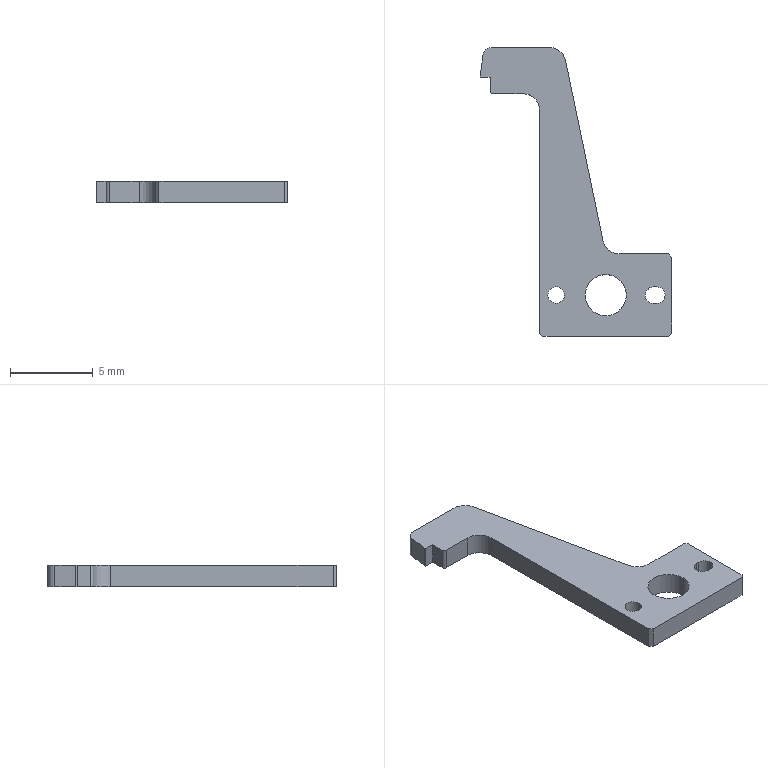Part | SolidWorks | features ICE 4, Fillet 3, Chamfer 1, Extrusion 1 | 1 solid | 30 faces | box 11.6 x 17.5 x 1.3 mm | volume 99.407 mm3 | plane 18 | cylinder 12 | commonest cylinder face diameters 1 x6 2 x3 2.5 x2 0.4 x1
STEP:
#1=CARTESIAN_POINT('',(5.4,-6.25,-0.65));
#2=VERTEX_POINT('',#1);
#3=CARTESIAN_POINT('',(4.9,-5.75,-0.65));
#4=VERTEX_POINT('',#3);
#5=CARTESIAN_POINT('',(4.9,-6.25,-0.65));
#6=DIRECTION('',(0.,0.,1.));
#7=DIRECTION('',(1.,0.,0.));
#8=AXIS2_PLACEMENT_3D('',#5,#6,#7);
#9=CIRCLE('',#8,0.5);
#10=EDGE_CURVE('',#2,#4,#9,.T.);
#11=ORIENTED_EDGE('',*,*,#10,.F.);
#12=CARTESIAN_POINT('',(5.4,-6.25,0.65));
#13=VERTEX_POINT('',#12);
#14=CARTESIAN_POINT('',(5.4,-6.25,-0.65));
#15=DIRECTION('',(0.,0.,1.));
#16=VECTOR('',#15,1000.);
#17=LINE('',#14,#16);
#18=EDGE_CURVE('',#2,#13,#17,.T.);
#19=ORIENTED_EDGE('',*,*,#18,.T.);
#20=CARTESIAN_POINT('',(4.9,-5.75,0.65));
#21=VERTEX_POINT('',#20);
#22=CARTESIAN_POINT('',(4.9,-6.25,0.65));
#23=DIRECTION('',(0.,0.,1.));
#24=DIRECTION('',(1.,0.,0.));
#25=AXIS2_PLACEMENT_3D('',#22,#23,#24);
#26=CIRCLE('',#25,0.5);
#27=EDGE_CURVE('',#13,#21,#26,.T.);
#28=ORIENTED_EDGE('',*,*,#27,.T.);
#29=CARTESIAN_POINT('',(4.9,-5.75,-0.65));
#30=DIRECTION('',(0.,0.,1.));
#31=VECTOR('',#30,1000.);
#32=LINE('',#29,#31);
#33=EDGE_CURVE('',#4,#21,#32,.T.);
#34=ORIENTED_EDGE('',*,*,#33,.F.);
#35=EDGE_LOOP('',(#11,#19,#28,#34));
#36=FACE_OUTER_BOUND('',#35,.T.);
#37=CARTESIAN_POINT('',(4.9,-6.25,-0.65));
#38=DIRECTION('',(0.,0.,1.));
#39=DIRECTION('',(1.,0.,0.));
#40=AXIS2_PLACEMENT_3D('',#37,#38,#39);
#41=CYLINDRICAL_SURFACE('',#40,0.5);
#42=ADVANCED_FACE('',(#36),#41,.F.);
#43=CARTESIAN_POINT('',(-1.7,-6.25,-0.65));
#44=VERTEX_POINT('',#43);
#45=CARTESIAN_POINT('',(-0.7,-6.25,-0.65));
#46=VERTEX_POINT('',#45);
#47=CARTESIAN_POINT('',(-1.2,-6.25,-0.65));
#48=DIRECTION('',(0.,0.,1.));
#49=DIRECTION('',(1.,0.,0.));
#50=AXIS2_PLACEMENT_3D('',#47,#48,#49);
#51=CIRCLE('',#50,0.5);
#52=EDGE_CURVE('',#44,#46,#51,.T.);
#53=ORIENTED_EDGE('',*,*,#52,.F.);
#54=CARTESIAN_POINT('',(-1.7,-6.25,0.65));
#55=VERTEX_POINT('',#54);
#56=CARTESIAN_POINT('',(-1.7,-6.25,-0.65));
#57=DIRECTION('',(0.,0.,1.));
#58=VECTOR('',#57,1000.);
#59=LINE('',#56,#58);
#60=EDGE_CURVE('',#44,#55,#59,.T.);
#61=ORIENTED_EDGE('',*,*,#60,.T.);
#62=CARTESIAN_POINT('',(-0.7,-6.25,0.65));
#63=VERTEX_POINT('',#62);
#64=CARTESIAN_POINT('',(-1.2,-6.25,0.65));
#65=DIRECTION('',(0.,0.,1.));
#66=DIRECTION('',(1.,0.,0.));
#67=AXIS2_PLACEMENT_3D('',#64,#65,#66);
#68=CIRCLE('',#67,0.5);
#69=EDGE_CURVE('',#55,#63,#68,.T.);
#70=ORIENTED_EDGE('',*,*,#69,.T.);
#71=CARTESIAN_POINT('',(-0.7,-6.25,-0.65));
#72=DIRECTION('',(0.,0.,1.));
#73=VECTOR('',#72,1000.);
#74=LINE('',#71,#73);
#75=EDGE_CURVE('',#46,#63,#74,.T.);
#76=ORIENTED_EDGE('',*,*,#75,.F.);
#77=EDGE_LOOP('',(#53,#61,#70,#76));
#78=FACE_OUTER_BOUND('',#77,.T.);
#79=CARTESIAN_POINT('',(-1.2,-6.25,-0.65));
#80=DIRECTION('',(0.,0.,1.));
#81=DIRECTION('',(1.,0.,0.));
#82=AXIS2_PLACEMENT_3D('',#79,#80,#81);
#83=CYLINDRICAL_SURFACE('',#82,0.5);
#84=ADVANCED_FACE('',(#78),#83,.F.);
#85=CARTESIAN_POINT('',(0.55,-6.25,-0.65));
#86=VERTEX_POINT('',#85);
#87=CARTESIAN_POINT('',(3.05,-6.25,-0.65));
#88=VERTEX_POINT('',#87);
#89=CARTESIAN_POINT('',(1.8,-6.25,-0.65));
#90=DIRECTION('',(0.,0.,1.));
#91=DIRECTION('',(1.,0.,0.));
#92=AXIS2_PLACEMENT_3D('',#89,#90,#91);
#93=CIRCLE('',#92,1.25);
#94=EDGE_CURVE('',#86,#88,#93,.T.);
#95=ORIENTED_EDGE('',*,*,#94,.F.);
#96=CARTESIAN_POINT('',(0.55,-6.25,0.65));
#97=VERTEX_POINT('',#96);
#98=CARTESIAN_POINT('',(0.55,-6.25,-0.65));
#99=DIRECTION('',(0.,0.,1.));
#100=VECTOR('',#99,1000.);
#101=LINE('',#98,#100);
#102=EDGE_CURVE('',#86,#97,#101,.T.);
#103=ORIENTED_EDGE('',*,*,#102,.T.);
#104=CARTESIAN_POINT('',(3.05,-6.25,0.65));
#105=VERTEX_POINT('',#104);
#106=CARTESIAN_POINT('',(1.8,-6.25,0.65));
#107=DIRECTION('',(0.,0.,1.));
#108=DIRECTION('',(1.,0.,0.));
#109=AXIS2_PLACEMENT_3D('',#106,#107,#108);
#110=CIRCLE('',#109,1.25);
#111=EDGE_CURVE('',#97,#105,#110,.T.);
#112=ORIENTED_EDGE('',*,*,#111,.T.);
#113=CARTESIAN_POINT('',(3.05,-6.25,-0.65));
#114=DIRECTION('',(0.,0.,1.));
#115=VECTOR('',#114,1000.);
#116=LINE('',#113,#115);
#117=EDGE_CURVE('',#88,#105,#116,.T.);
#118=ORIENTED_EDGE('',*,*,#117,.F.);
#119=EDGE_LOOP('',(#95,#103,#112,#118));
#120=FACE_OUTER_BOUND('',#119,.T.);
#121=CARTESIAN_POINT('',(1.8,-6.25,-0.65));
#122=DIRECTION('',(0.,0.,1.));
#123=DIRECTION('',(1.,0.,0.));
#124=AXIS2_PLACEMENT_3D('',#121,#122,#123);
#125=CYLINDRICAL_SURFACE('',#124,1.25);
#126=ADVANCED_FACE('',(#120),#125,.F.);
#127=CARTESIAN_POINT('',(5.8,-8.55,-0.65));
#128=VERTEX_POINT('',#127);
#129=CARTESIAN_POINT('',(5.8,-3.95,-0.65));
#130=VERTEX_POINT('',#129);
#131=CARTESIAN_POINT('',(5.8,8.75,-0.65));
#132=DIRECTION('',(0.,1.,0.));
#133=VECTOR('',#132,1000.);
#134=LINE('',#131,#133);
#135=EDGE_CURVE('',#128,#130,#134,.T.);
#136=ORIENTED_EDGE('',*,*,#135,.T.);
#137=CARTESIAN_POINT('',(5.8,-3.95,0.65));
#138=VERTEX_POINT('',#137);
#139=CARTESIAN_POINT('',(5.8,-3.95,0.65));
#140=DIRECTION('',(0.,0.,1.));
#141=VECTOR('',#140,1000.);
#142=LINE('',#139,#141);
#143=EDGE_CURVE('',#130,#138,#142,.T.);
#144=ORIENTED_EDGE('',*,*,#143,.T.);
#145=CARTESIAN_POINT('',(5.8,-8.55,0.65));
#146=VERTEX_POINT('',#145);
#147=CARTESIAN_POINT('',(5.8,8.75,0.65));
#148=DIRECTION('',(0.,1.,0.));
#149=VECTOR('',#148,1000.);
#150=LINE('',#147,#149);
#151=EDGE_CURVE('',#146,#138,#150,.T.);
#152=ORIENTED_EDGE('',*,*,#151,.F.);
#153=CARTESIAN_POINT('',(5.8,-8.55,0.65));
#154=DIRECTION('',(0.,0.,-1.));
#155=VECTOR('',#154,1000.);
#156=LINE('',#153,#155);
#157=EDGE_CURVE('',#146,#128,#156,.T.);
#158=ORIENTED_EDGE('',*,*,#157,.T.);
#159=EDGE_LOOP('',(#136,#144,#152,#158));
#160=FACE_OUTER_BOUND('',#159,.T.);
#161=CARTESIAN_POINT('',(5.8,8.75,0.65));
#162=DIRECTION('',(-1.,0.,0.));
#163=DIRECTION('',(0.,-1.,0.));
#164=AXIS2_PLACEMENT_3D('',#161,#162,#163);
#165=PLANE('',#164);
#166=ADVANCED_FACE('',(#160),#165,.F.);
#167=CARTESIAN_POINT('',(-1.613,8.75,-0.65));
#168=VERTEX_POINT('',#167);
#169=CARTESIAN_POINT('',(-5.138,8.75,-0.65));
#170=VERTEX_POINT('',#169);
#171=CARTESIAN_POINT('',(-5.8,8.75,-0.65));
#172=DIRECTION('',(-1.,0.,0.));
#173=VECTOR('',#172,1000.);
#174=LINE('',#171,#173);
#175=EDGE_CURVE('',#168,#170,#174,.T.);
#176=ORIENTED_EDGE('',*,*,#175,.T.);
#177=CARTESIAN_POINT('',(-5.138,8.75,0.65));
#178=VERTEX_POINT('',#177);
#179=CARTESIAN_POINT('',(-5.138,8.75,0.65));
#180=DIRECTION('',(0.,0.,1.));
#181=VECTOR('',#180,1000.);
#182=LINE('',#179,#181);
#183=EDGE_CURVE('',#170,#178,#182,.T.);
#184=ORIENTED_EDGE('',*,*,#183,.T.);
#185=CARTESIAN_POINT('',(-1.613,8.75,0.65));
#186=VERTEX_POINT('',#185);
#187=CARTESIAN_POINT('',(-5.8,8.75,0.65));
#188=DIRECTION('',(-1.,0.,0.));
#189=VECTOR('',#188,1000.);
#190=LINE('',#187,#189);
#191=EDGE_CURVE('',#186,#178,#190,.T.);
#192=ORIENTED_EDGE('',*,*,#191,.F.);
#193=CARTESIAN_POINT('',(-1.613,8.75,0.65));
#194=DIRECTION('',(0.,0.,-1.));
#195=VECTOR('',#194,1000.);
#196=LINE('',#193,#195);
#197=EDGE_CURVE('',#186,#168,#196,.T.);
#198=ORIENTED_EDGE('',*,*,#197,.T.);
#199=EDGE_LOOP('',(#176,#184,#192,#198));
#200=FACE_OUTER_BOUND('',#199,.T.);
#201=CARTESIAN_POINT('',(-5.8,8.75,0.65));
#202=DIRECTION('',(0.,-1.,0.));
#203=DIRECTION('',(0.,0.,-1.));
#204=AXIS2_PLACEMENT_3D('',#201,#202,#203);
#205=PLANE('',#204);
#206=ADVANCED_FACE('',(#200),#205,.F.);
#207=CARTESIAN_POINT('',(-5.8,7.05,0.65));
#208=VERTEX_POINT('',#207);
#209=CARTESIAN_POINT('',(-5.8,6.95,0.65));
#210=VERTEX_POINT('',#209);
#211=CARTESIAN_POINT('',(-5.8,8.75,0.65));
#212=DIRECTION('',(0.,-1.,0.));
#213=VECTOR('',#212,1000.);
#214=LINE('',#211,#213);
#215=EDGE_CURVE('',#208,#210,#214,.T.);
#216=ORIENTED_EDGE('',*,*,#215,.F.);
#217=CARTESIAN_POINT('',(-5.8,7.05,-0.65));
#218=VERTEX_POINT('',#217);
#219=CARTESIAN_POINT('',(-5.8,7.05,-0.65));
#220=DIRECTION('',(0.,0.,1.));
#221=VECTOR('',#220,1000.);
#222=LINE('',#219,#221);
#223=EDGE_CURVE('',#218,#208,#222,.T.);
#224=ORIENTED_EDGE('',*,*,#223,.F.);
#225=CARTESIAN_POINT('',(-5.8,6.95,-0.65));
#226=VERTEX_POINT('',#225);
#227=CARTESIAN_POINT('',(-5.8,8.75,-0.65));
#228=DIRECTION('',(0.,-1.,0.));
#229=VECTOR('',#228,1000.);
#230=LINE('',#227,#229);
#231=EDGE_CURVE('',#218,#226,#230,.T.);
#232=ORIENTED_EDGE('',*,*,#231,.T.);
#233=CARTESIAN_POINT('',(-5.8,6.95,-0.65));
#234=DIRECTION('',(0.,0.,1.));
#235=VECTOR('',#234,1000.);
#236=LINE('',#233,#235);
#237=EDGE_CURVE('',#226,#210,#236,.T.);
#238=ORIENTED_EDGE('',*,*,#237,.T.);
#239=EDGE_LOOP('',(#216,#224,#232,#238));
#240=FACE_OUTER_BOUND('',#239,.T.);
#241=CARTESIAN_POINT('',(-5.8,8.75,0.65));
#242=DIRECTION('',(1.,0.,0.));
#243=DIRECTION('',(0.,1.,0.));
#244=AXIS2_PLACEMENT_3D('',#241,#242,#243);
#245=PLANE('',#244);
#246=ADVANCED_FACE('',(#240),#245,.F.);
#247=CARTESIAN_POINT('',(-2.,-8.75,-0.65));
#248=VERTEX_POINT('',#247);
#249=CARTESIAN_POINT('',(5.6,-8.75,-0.65));
#250=VERTEX_POINT('',#249);
#251=CARTESIAN_POINT('',(-5.8,-8.75,-0.65));
#252=DIRECTION('',(1.,0.,0.));
#253=VECTOR('',#252,1000.);
#254=LINE('',#251,#253);
#255=EDGE_CURVE('',#248,#250,#254,.T.);
#256=ORIENTED_EDGE('',*,*,#255,.T.);
#257=CARTESIAN_POINT('',(5.6,-8.75,0.65));
#258=VERTEX_POINT('',#257);
#259=CARTESIAN_POINT('',(5.6,-8.75,0.65));
#260=DIRECTION('',(0.,0.,1.));
#261=VECTOR('',#260,1000.);
#262=LINE('',#259,#261);
#263=EDGE_CURVE('',#250,#258,#262,.T.);
#264=ORIENTED_EDGE('',*,*,#263,.T.);
#265=CARTESIAN_POINT('',(-2.,-8.75,0.65));
#266=VERTEX_POINT('',#265);
#267=CARTESIAN_POINT('',(-5.8,-8.75,0.65));
#268=DIRECTION('',(1.,0.,0.));
#269=VECTOR('',#268,1000.);
#270=LINE('',#267,#269);
#271=EDGE_CURVE('',#266,#258,#270,.T.);
#272=ORIENTED_EDGE('',*,*,#271,.F.);
#273=CARTESIAN_POINT('',(-2.,-8.75,0.65));
#274=DIRECTION('',(0.,0.,-1.));
#275=VECTOR('',#274,1000.);
#276=LINE('',#273,#275);
#277=EDGE_CURVE('',#266,#248,#276,.T.);
#278=ORIENTED_EDGE('',*,*,#277,.T.);
#279=EDGE_LOOP('',(#256,#264,#272,#278));
#280=FACE_OUTER_BOUND('',#279,.T.);
#281=CARTESIAN_POINT('',(-5.8,-8.75,0.65));
#282=DIRECTION('',(0.,1.,0.));
#283=DIRECTION('',(0.,0.,1.));
#284=AXIS2_PLACEMENT_3D('',#281,#282,#283);
#285=PLANE('',#284);
#286=ADVANCED_FACE('',(#280),#285,.F.);
#287=ORIENTED_EDGE('',*,*,#191,.T.);
#288=CARTESIAN_POINT('',(-5.633,8.315,0.65));
#289=VERTEX_POINT('',#288);
#290=CARTESIAN_POINT('',(-5.138,8.25,0.65));
#291=DIRECTION('',(0.,0.,1.));
#292=DIRECTION('',(1.,0.,0.));
#293=AXIS2_PLACEMENT_3D('',#290,#291,#292);
#294=CIRCLE('',#293,0.5);
#295=EDGE_CURVE('',#178,#289,#294,.T.);
#296=ORIENTED_EDGE('',*,*,#295,.T.);
#297=CARTESIAN_POINT('',(-5.8,7.05,0.65));
#298=DIRECTION('',(0.1305,0.9914,0.));
#299=VECTOR('',#298,1000.);
#300=LINE('',#297,#299);
#301=EDGE_CURVE('',#208,#289,#300,.T.);
#302=ORIENTED_EDGE('',*,*,#301,.F.);
#303=ORIENTED_EDGE('',*,*,#215,.T.);
#304=CARTESIAN_POINT('',(-5.2,6.95,0.65));
#305=VERTEX_POINT('',#304);
#306=CARTESIAN_POINT('',(-5.8,6.95,0.65));
#307=DIRECTION('',(-1.,0.,0.));
#308=VECTOR('',#307,1000.);
#309=LINE('',#306,#308);
#310=EDGE_CURVE('',#305,#210,#309,.T.);
#311=ORIENTED_EDGE('',*,*,#310,.F.);
#312=CARTESIAN_POINT('',(-5.2,6.15,0.65));
#313=VERTEX_POINT('',#312);
#314=CARTESIAN_POINT('',(-5.2,5.95,0.65));
#315=DIRECTION('',(0.,1.,0.));
#316=VECTOR('',#315,1000.);
#317=LINE('',#314,#316);
#318=EDGE_CURVE('',#313,#305,#317,.T.);
#319=ORIENTED_EDGE('',*,*,#318,.F.);
#320=CARTESIAN_POINT('',(-5.,5.95,0.65));
#321=VERTEX_POINT('',#320);
#322=CARTESIAN_POINT('',(-5.,6.15,0.65));
#323=DIRECTION('',(0.,0.,1.));
#324=DIRECTION('',(1.,0.,0.));
#325=AXIS2_PLACEMENT_3D('',#322,#323,#324);
#326=CIRCLE('',#325,0.2);
#327=EDGE_CURVE('',#313,#321,#326,.T.);
#328=ORIENTED_EDGE('',*,*,#327,.T.);
#329=CARTESIAN_POINT('',(-3.2,5.95,0.65));
#330=VERTEX_POINT('',#329);
#331=CARTESIAN_POINT('',(-5.8,5.95,0.65));
#332=DIRECTION('',(-1.,0.,0.));
#333=VECTOR('',#332,1000.);
#334=LINE('',#331,#333);
#335=EDGE_CURVE('',#330,#321,#334,.T.);
#336=ORIENTED_EDGE('',*,*,#335,.F.);
#337=CARTESIAN_POINT('',(-2.2,4.95,0.65));
#338=VERTEX_POINT('',#337);
#339=CARTESIAN_POINT('',(-3.2,4.95,0.65));
#340=DIRECTION('',(0.,0.,-1.));
#341=DIRECTION('',(1.,0.,0.));
#342=AXIS2_PLACEMENT_3D('',#339,#340,#341);
#343=CIRCLE('',#342,1.);
#344=EDGE_CURVE('',#330,#338,#343,.T.);
#345=ORIENTED_EDGE('',*,*,#344,.T.);
#346=CARTESIAN_POINT('',(-2.2,-8.55,0.65));
#347=VERTEX_POINT('',#346);
#348=CARTESIAN_POINT('',(-2.2,-8.75,0.65));
#349=DIRECTION('',(0.,1.,0.));
#350=VECTOR('',#349,1000.);
#351=LINE('',#348,#350);
#352=EDGE_CURVE('',#347,#338,#351,.T.);
#353=ORIENTED_EDGE('',*,*,#352,.F.);
#354=CARTESIAN_POINT('',(-5.375,-5.375,0.65));
#355=DIRECTION('',(0.7071,-0.7071,0.));
#356=VECTOR('',#355,1000.);
#357=LINE('',#354,#356);
#358=EDGE_CURVE('',#347,#266,#357,.T.);
#359=ORIENTED_EDGE('',*,*,#358,.T.);
#360=ORIENTED_EDGE('',*,*,#271,.T.);
#361=CARTESIAN_POINT('',(7.175,-7.175,0.65));
#362=DIRECTION('',(0.7071,0.7071,0.));
#363=VECTOR('',#362,1000.);
#364=LINE('',#361,#363);
#365=EDGE_CURVE('',#258,#146,#364,.T.);
#366=ORIENTED_EDGE('',*,*,#365,.T.);
#367=ORIENTED_EDGE('',*,*,#151,.T.);
#368=CARTESIAN_POINT('',(5.6,-3.75,0.65));
#369=VERTEX_POINT('',#368);
#370=CARTESIAN_POINT('',(0.925,0.925,0.65));
#371=DIRECTION('',(-0.7071,0.7071,0.));
#372=VECTOR('',#371,1000.);
#373=LINE('',#370,#372);
#374=EDGE_CURVE('',#138,#369,#373,.T.);
#375=ORIENTED_EDGE('',*,*,#374,.T.);
#376=CARTESIAN_POINT('',(2.613,-3.75,0.65));
#377=VERTEX_POINT('',#376);
#378=CARTESIAN_POINT('',(5.8,-3.75,0.65));
#379=DIRECTION('',(1.,0.,0.));
#380=VECTOR('',#379,1000.);
#381=LINE('',#378,#380);
#382=EDGE_CURVE('',#377,#369,#381,.T.);
#383=ORIENTED_EDGE('',*,*,#382,.F.);
#384=CARTESIAN_POINT('',(1.634,-2.954,0.65));
#385=VERTEX_POINT('',#384);
#386=CARTESIAN_POINT('',(2.613,-2.75,0.65));
#387=DIRECTION('',(0.,0.,-1.));
#388=DIRECTION('',(1.,0.,0.));
#389=AXIS2_PLACEMENT_3D('',#386,#387,#388);
#390=CIRCLE('',#389,1.);
#391=EDGE_CURVE('',#377,#385,#390,.T.);
#392=ORIENTED_EDGE('',*,*,#391,.T.);
#393=CARTESIAN_POINT('',(-0.6344,7.954,0.65));
#394=VERTEX_POINT('',#393);
#395=CARTESIAN_POINT('',(1.8,-3.75,0.65));
#396=DIRECTION('',(0.2036,-0.979,0.));
#397=VECTOR('',#396,1000.);
#398=LINE('',#395,#397);
#399=EDGE_CURVE('',#394,#385,#398,.T.);
#400=ORIENTED_EDGE('',*,*,#399,.F.);
#401=CARTESIAN_POINT('',(-1.613,7.75,0.65));
#402=DIRECTION('',(0.,0.,1.));
#403=DIRECTION('',(1.,0.,0.));
#404=AXIS2_PLACEMENT_3D('',#401,#402,#403);
#405=CIRCLE('',#404,1.);
#406=EDGE_CURVE('',#394,#186,#405,.T.);
#407=ORIENTED_EDGE('',*,*,#406,.T.);
#408=EDGE_LOOP('',(#287,#296,#302,#303,#311,#319,#328,#336,#345,#353,#359,#360,#366,#367,#375,#383,#392,#400,#407));
#409=FACE_OUTER_BOUND('',#408,.T.);
#410=CARTESIAN_POINT('',(4.7,-5.75,0.65));
#411=VERTEX_POINT('',#410);
#412=CARTESIAN_POINT('',(4.7,-6.75,0.65));
#413=VERTEX_POINT('',#412);
#414=CARTESIAN_POINT('',(4.7,-6.25,0.65));
#415=DIRECTION('',(0.,0.,1.));
#416=DIRECTION('',(1.,0.,0.));
#417=AXIS2_PLACEMENT_3D('',#414,#415,#416);
#418=CIRCLE('',#417,0.5);
#419=EDGE_CURVE('',#411,#413,#418,.T.);
#420=ORIENTED_EDGE('',*,*,#419,.F.);
#421=CARTESIAN_POINT('',(4.7,-5.75,0.65));
#422=DIRECTION('',(-1.,0.,0.));
#423=VECTOR('',#422,1000.);
#424=LINE('',#421,#423);
#425=EDGE_CURVE('',#21,#411,#424,.T.);
#426=ORIENTED_EDGE('',*,*,#425,.F.);
#427=ORIENTED_EDGE('',*,*,#27,.F.);
#428=CARTESIAN_POINT('',(4.9,-6.75,0.65));
#429=VERTEX_POINT('',#428);
#430=CARTESIAN_POINT('',(4.9,-6.25,0.65));
#431=DIRECTION('',(0.,0.,1.));
#432=DIRECTION('',(1.,0.,0.));
#433=AXIS2_PLACEMENT_3D('',#430,#431,#432);
#434=CIRCLE('',#433,0.5);
#435=EDGE_CURVE('',#429,#13,#434,.T.);
#436=ORIENTED_EDGE('',*,*,#435,.F.);
#437=CARTESIAN_POINT('',(4.7,-6.75,0.65));
#438=DIRECTION('',(1.,0.,0.));
#439=VECTOR('',#438,1000.);
#440=LINE('',#437,#439);
#441=EDGE_CURVE('',#413,#429,#440,.T.);
#442=ORIENTED_EDGE('',*,*,#441,.F.);
#443=EDGE_LOOP('',(#420,#426,#427,#436,#442));
#444=FACE_BOUND('',#443,.T.);
#445=CARTESIAN_POINT('',(-1.2,-6.25,0.65));
#446=DIRECTION('',(0.,0.,1.));
#447=DIRECTION('',(1.,0.,0.));
#448=AXIS2_PLACEMENT_3D('',#445,#446,#447);
#449=CIRCLE('',#448,0.5);
#450=EDGE_CURVE('',#63,#55,#449,.T.);
#451=ORIENTED_EDGE('',*,*,#450,.F.);
#452=ORIENTED_EDGE('',*,*,#69,.F.);
#453=EDGE_LOOP('',(#451,#452));
#454=FACE_BOUND('',#453,.T.);
#455=CARTESIAN_POINT('',(1.8,-6.25,0.65));
#456=DIRECTION('',(0.,0.,1.));
#457=DIRECTION('',(1.,0.,0.));
#458=AXIS2_PLACEMENT_3D('',#455,#456,#457);
#459=CIRCLE('',#458,1.25);
#460=EDGE_CURVE('',#105,#97,#459,.T.);
#461=ORIENTED_EDGE('',*,*,#460,.F.);
#462=ORIENTED_EDGE('',*,*,#111,.F.);
#463=EDGE_LOOP('',(#461,#462));
#464=FACE_BOUND('',#463,.T.);
#465=CARTESIAN_POINT('',(0.,0.,0.65));
#466=DIRECTION('',(0.,0.,1.));
#467=DIRECTION('',(1.,0.,0.));
#468=AXIS2_PLACEMENT_3D('',#465,#466,#467);
#469=PLANE('',#468);
#470=ADVANCED_FACE('',(#409,#444,#454,#464),#469,.T.);
#471=CARTESIAN_POINT('',(4.7,-5.75,-0.65));
#472=VERTEX_POINT('',#471);
#473=CARTESIAN_POINT('',(4.7,-5.75,-0.65));
#474=DIRECTION('',(-1.,0.,0.));
#475=VECTOR('',#474,1000.);
#476=LINE('',#473,#475);
#477=EDGE_CURVE('',#4,#472,#476,.T.);
#478=ORIENTED_EDGE('',*,*,#477,.T.);
#479=CARTESIAN_POINT('',(4.7,-6.75,-0.65));
#480=VERTEX_POINT('',#479);
#481=CARTESIAN_POINT('',(4.7,-6.25,-0.65));
#482=DIRECTION('',(0.,0.,1.));
#483=DIRECTION('',(1.,0.,0.));
#484=AXIS2_PLACEMENT_3D('',#481,#482,#483);
#485=CIRCLE('',#484,0.5);
#486=EDGE_CURVE('',#472,#480,#485,.T.);
#487=ORIENTED_EDGE('',*,*,#486,.T.);
#488=CARTESIAN_POINT('',(4.9,-6.75,-0.65));
#489=VERTEX_POINT('',#488);
#490=CARTESIAN_POINT('',(4.7,-6.75,-0.65));
#491=DIRECTION('',(1.,0.,0.));
#492=VECTOR('',#491,1000.);
#493=LINE('',#490,#492);
#494=EDGE_CURVE('',#480,#489,#493,.T.);
#495=ORIENTED_EDGE('',*,*,#494,.T.);
#496=CARTESIAN_POINT('',(4.9,-6.25,-0.65));
#497=DIRECTION('',(0.,0.,1.));
#498=DIRECTION('',(1.,0.,0.));
#499=AXIS2_PLACEMENT_3D('',#496,#497,#498);
#500=CIRCLE('',#499,0.5);
#501=EDGE_CURVE('',#489,#2,#500,.T.);
#502=ORIENTED_EDGE('',*,*,#501,.T.);
#503=ORIENTED_EDGE('',*,*,#10,.T.);
#504=EDGE_LOOP('',(#478,#487,#495,#502,#503));
#505=FACE_BOUND('',#504,.T.);
#506=CARTESIAN_POINT('',(-1.2,-6.25,-0.65));
#507=DIRECTION('',(0.,0.,1.));
#508=DIRECTION('',(1.,0.,0.));
#509=AXIS2_PLACEMENT_3D('',#506,#507,#508);
#510=CIRCLE('',#509,0.5);
#511=EDGE_CURVE('',#46,#44,#510,.T.);
#512=ORIENTED_EDGE('',*,*,#511,.T.);
#513=ORIENTED_EDGE('',*,*,#52,.T.);
#514=EDGE_LOOP('',(#512,#513));
#515=FACE_BOUND('',#514,.T.);
#516=CARTESIAN_POINT('',(1.8,-6.25,-0.65));
#517=DIRECTION('',(0.,0.,1.));
#518=DIRECTION('',(1.,0.,0.));
#519=AXIS2_PLACEMENT_3D('',#516,#517,#518);
#520=CIRCLE('',#519,1.25);
#521=EDGE_CURVE('',#88,#86,#520,.T.);
#522=ORIENTED_EDGE('',*,*,#521,.T.);
#523=ORIENTED_EDGE('',*,*,#94,.T.);
#524=EDGE_LOOP('',(#522,#523));
#525=FACE_BOUND('',#524,.T.);
#526=CARTESIAN_POINT('',(-5.633,8.315,-0.65));
#527=VERTEX_POINT('',#526);
#528=CARTESIAN_POINT('',(-5.8,7.05,-0.65));
#529=DIRECTION('',(0.1305,0.9914,0.));
#530=VECTOR('',#529,1000.);
#531=LINE('',#528,#530);
#532=EDGE_CURVE('',#218,#527,#531,.T.);
#533=ORIENTED_EDGE('',*,*,#532,.T.);
#534=CARTESIAN_POINT('',(-5.138,8.25,-0.65));
#535=DIRECTION('',(0.,0.,-1.));
#536=DIRECTION('',(1.,0.,0.));
#537=AXIS2_PLACEMENT_3D('',#534,#535,#536);
#538=CIRCLE('',#537,0.5);
#539=EDGE_CURVE('',#527,#170,#538,.T.);
#540=ORIENTED_EDGE('',*,*,#539,.T.);
#541=ORIENTED_EDGE('',*,*,#175,.F.);
#542=CARTESIAN_POINT('',(-0.6344,7.954,-0.65));
#543=VERTEX_POINT('',#542);
#544=CARTESIAN_POINT('',(-1.613,7.75,-0.65));
#545=DIRECTION('',(0.,0.,-1.));
#546=DIRECTION('',(1.,0.,0.));
#547=AXIS2_PLACEMENT_3D('',#544,#545,#546);
#548=CIRCLE('',#547,1.);
#549=EDGE_CURVE('',#168,#543,#548,.T.);
#550=ORIENTED_EDGE('',*,*,#549,.T.);
#551=CARTESIAN_POINT('',(1.634,-2.954,-0.65));
#552=VERTEX_POINT('',#551);
#553=CARTESIAN_POINT('',(1.8,-3.75,-0.65));
#554=DIRECTION('',(0.2036,-0.979,0.));
#555=VECTOR('',#554,1000.);
#556=LINE('',#553,#555);
#557=EDGE_CURVE('',#543,#552,#556,.T.);
#558=ORIENTED_EDGE('',*,*,#557,.T.);
#559=CARTESIAN_POINT('',(2.613,-3.75,-0.65));
#560=VERTEX_POINT('',#559);
#561=CARTESIAN_POINT('',(2.613,-2.75,-0.65));
#562=DIRECTION('',(0.,0.,1.));
#563=DIRECTION('',(1.,0.,0.));
#564=AXIS2_PLACEMENT_3D('',#561,#562,#563);
#565=CIRCLE('',#564,1.);
#566=EDGE_CURVE('',#552,#560,#565,.T.);
#567=ORIENTED_EDGE('',*,*,#566,.T.);
#568=CARTESIAN_POINT('',(5.6,-3.75,-0.65));
#569=VERTEX_POINT('',#568);
#570=CARTESIAN_POINT('',(5.8,-3.75,-0.65));
#571=DIRECTION('',(1.,0.,0.));
#572=VECTOR('',#571,1000.);
#573=LINE('',#570,#572);
#574=EDGE_CURVE('',#560,#569,#573,.T.);
#575=ORIENTED_EDGE('',*,*,#574,.T.);
#576=CARTESIAN_POINT('',(5.8,-3.95,-0.65));
#577=DIRECTION('',(0.7071,-0.7071,0.));
#578=VECTOR('',#577,1000.);
#579=LINE('',#576,#578);
#580=EDGE_CURVE('',#569,#130,#579,.T.);
#581=ORIENTED_EDGE('',*,*,#580,.T.);
#582=ORIENTED_EDGE('',*,*,#135,.F.);
#583=CARTESIAN_POINT('',(5.8,-8.55,-0.65));
#584=DIRECTION('',(-0.7071,-0.7071,0.));
#585=VECTOR('',#584,1000.);
#586=LINE('',#583,#585);
#587=EDGE_CURVE('',#128,#250,#586,.T.);
#588=ORIENTED_EDGE('',*,*,#587,.T.);
#589=ORIENTED_EDGE('',*,*,#255,.F.);
#590=CARTESIAN_POINT('',(-2.2,-8.55,-0.65));
#591=VERTEX_POINT('',#590);
#592=CARTESIAN_POINT('',(-2.2,-8.55,-0.65));
#593=DIRECTION('',(-0.7071,0.7071,0.));
#594=VECTOR('',#593,1000.);
#595=LINE('',#592,#594);
#596=EDGE_CURVE('',#248,#591,#595,.T.);
#597=ORIENTED_EDGE('',*,*,#596,.T.);
#598=CARTESIAN_POINT('',(-2.2,4.95,-0.65));
#599=VERTEX_POINT('',#598);
#600=CARTESIAN_POINT('',(-2.2,-8.75,-0.65));
#601=DIRECTION('',(0.,1.,0.));
#602=VECTOR('',#601,1000.);
#603=LINE('',#600,#602);
#604=EDGE_CURVE('',#591,#599,#603,.T.);
#605=ORIENTED_EDGE('',*,*,#604,.T.);
#606=CARTESIAN_POINT('',(-3.2,5.95,-0.65));
#607=VERTEX_POINT('',#606);
#608=CARTESIAN_POINT('',(-3.2,4.95,-0.65));
#609=DIRECTION('',(0.,0.,1.));
#610=DIRECTION('',(1.,0.,0.));
#611=AXIS2_PLACEMENT_3D('',#608,#609,#610);
#612=CIRCLE('',#611,1.);
#613=EDGE_CURVE('',#599,#607,#612,.T.);
#614=ORIENTED_EDGE('',*,*,#613,.T.);
#615=CARTESIAN_POINT('',(-5.,5.95,-0.65));
#616=VERTEX_POINT('',#615);
#617=CARTESIAN_POINT('',(-5.8,5.95,-0.65));
#618=DIRECTION('',(-1.,0.,0.));
#619=VECTOR('',#618,1000.);
#620=LINE('',#617,#619);
#621=EDGE_CURVE('',#607,#616,#620,.T.);
#622=ORIENTED_EDGE('',*,*,#621,.T.);
#623=CARTESIAN_POINT('',(-5.2,6.15,-0.65));
#624=VERTEX_POINT('',#623);
#625=CARTESIAN_POINT('',(-5.,6.15,-0.65));
#626=DIRECTION('',(0.,0.,-1.));
#627=DIRECTION('',(1.,0.,0.));
#628=AXIS2_PLACEMENT_3D('',#625,#626,#627);
#629=CIRCLE('',#628,0.2);
#630=EDGE_CURVE('',#616,#624,#629,.T.);
#631=ORIENTED_EDGE('',*,*,#630,.T.);
#632=CARTESIAN_POINT('',(-5.2,6.95,-0.65));
#633=VERTEX_POINT('',#632);
#634=CARTESIAN_POINT('',(-5.2,5.95,-0.65));
#635=DIRECTION('',(0.,1.,0.));
#636=VECTOR('',#635,1000.);
#637=LINE('',#634,#636);
#638=EDGE_CURVE('',#624,#633,#637,.T.);
#639=ORIENTED_EDGE('',*,*,#638,.T.);
#640=CARTESIAN_POINT('',(-5.8,6.95,-0.65));
#641=DIRECTION('',(-1.,0.,0.));
#642=VECTOR('',#641,1000.);
#643=LINE('',#640,#642);
#644=EDGE_CURVE('',#633,#226,#643,.T.);
#645=ORIENTED_EDGE('',*,*,#644,.T.);
#646=ORIENTED_EDGE('',*,*,#231,.F.);
#647=EDGE_LOOP('',(#533,#540,#541,#550,#558,#567,#575,#581,#582,#588,#589,#597,#605,#614,#622,#631,#639,#645,#646));
#648=FACE_OUTER_BOUND('',#647,.T.);
#649=CARTESIAN_POINT('',(0.,0.,-0.65));
#650=DIRECTION('',(0.,0.,1.));
#651=DIRECTION('',(1.,0.,0.));
#652=AXIS2_PLACEMENT_3D('',#649,#650,#651);
#653=PLANE('',#652);
#654=ADVANCED_FACE('',(#505,#515,#525,#648),#653,.F.);
#655=ORIENTED_EDGE('',*,*,#102,.F.);
#656=ORIENTED_EDGE('',*,*,#521,.F.);
#657=ORIENTED_EDGE('',*,*,#117,.T.);
#658=ORIENTED_EDGE('',*,*,#460,.T.);
#659=EDGE_LOOP('',(#655,#656,#657,#658));
#660=FACE_OUTER_BOUND('',#659,.T.);
#661=CARTESIAN_POINT('',(1.8,-6.25,-0.65));
#662=DIRECTION('',(0.,0.,1.));
#663=DIRECTION('',(1.,0.,0.));
#664=AXIS2_PLACEMENT_3D('',#661,#662,#663);
#665=CYLINDRICAL_SURFACE('',#664,1.25);
#666=ADVANCED_FACE('',(#660),#665,.F.);
#667=ORIENTED_EDGE('',*,*,#60,.F.);
#668=ORIENTED_EDGE('',*,*,#511,.F.);
#669=ORIENTED_EDGE('',*,*,#75,.T.);
#670=ORIENTED_EDGE('',*,*,#450,.T.);
#671=EDGE_LOOP('',(#667,#668,#669,#670));
#672=FACE_OUTER_BOUND('',#671,.T.);
#673=CARTESIAN_POINT('',(-1.2,-6.25,-0.65));
#674=DIRECTION('',(0.,0.,1.));
#675=DIRECTION('',(1.,0.,0.));
#676=AXIS2_PLACEMENT_3D('',#673,#674,#675);
#677=CYLINDRICAL_SURFACE('',#676,0.5);
#678=ADVANCED_FACE('',(#672),#677,.F.);
#679=ORIENTED_EDGE('',*,*,#419,.T.);
#680=CARTESIAN_POINT('',(4.7,-6.75,-0.65));
#681=DIRECTION('',(0.,0.,1.));
#682=VECTOR('',#681,1000.);
#683=LINE('',#680,#682);
#684=EDGE_CURVE('',#480,#413,#683,.T.);
#685=ORIENTED_EDGE('',*,*,#684,.F.);
#686=ORIENTED_EDGE('',*,*,#486,.F.);
#687=CARTESIAN_POINT('',(4.7,-5.75,-0.65));
#688=DIRECTION('',(0.,0.,1.));
#689=VECTOR('',#688,1000.);
#690=LINE('',#687,#689);
#691=EDGE_CURVE('',#472,#411,#690,.T.);
#692=ORIENTED_EDGE('',*,*,#691,.T.);
#693=EDGE_LOOP('',(#679,#685,#686,#692));
#694=FACE_OUTER_BOUND('',#693,.T.);
#695=CARTESIAN_POINT('',(4.7,-6.25,-0.65));
#696=DIRECTION('',(0.,0.,1.));
#697=DIRECTION('',(1.,0.,0.));
#698=AXIS2_PLACEMENT_3D('',#695,#696,#697);
#699=CYLINDRICAL_SURFACE('',#698,0.5);
#700=ADVANCED_FACE('',(#694),#699,.F.);
#701=ORIENTED_EDGE('',*,*,#425,.T.);
#702=ORIENTED_EDGE('',*,*,#691,.F.);
#703=ORIENTED_EDGE('',*,*,#477,.F.);
#704=ORIENTED_EDGE('',*,*,#33,.T.);
#705=EDGE_LOOP('',(#701,#702,#703,#704));
#706=FACE_OUTER_BOUND('',#705,.T.);
#707=CARTESIAN_POINT('',(4.7,-5.75,-0.65));
#708=DIRECTION('',(0.,1.,0.));
#709=DIRECTION('',(0.,0.,1.));
#710=AXIS2_PLACEMENT_3D('',#707,#708,#709);
#711=PLANE('',#710);
#712=ADVANCED_FACE('',(#706),#711,.F.);
#713=ORIENTED_EDGE('',*,*,#18,.F.);
#714=ORIENTED_EDGE('',*,*,#501,.F.);
#715=CARTESIAN_POINT('',(4.9,-6.75,-0.65));
#716=DIRECTION('',(0.,0.,1.));
#717=VECTOR('',#716,1000.);
#718=LINE('',#715,#717);
#719=EDGE_CURVE('',#489,#429,#718,.T.);
#720=ORIENTED_EDGE('',*,*,#719,.T.);
#721=ORIENTED_EDGE('',*,*,#435,.T.);
#722=EDGE_LOOP('',(#713,#714,#720,#721));
#723=FACE_OUTER_BOUND('',#722,.T.);
#724=CARTESIAN_POINT('',(4.9,-6.25,-0.65));
#725=DIRECTION('',(0.,0.,1.));
#726=DIRECTION('',(1.,0.,0.));
#727=AXIS2_PLACEMENT_3D('',#724,#725,#726);
#728=CYLINDRICAL_SURFACE('',#727,0.5);
#729=ADVANCED_FACE('',(#723),#728,.F.);
#730=ORIENTED_EDGE('',*,*,#441,.T.);
#731=ORIENTED_EDGE('',*,*,#719,.F.);
#732=ORIENTED_EDGE('',*,*,#494,.F.);
#733=ORIENTED_EDGE('',*,*,#684,.T.);
#734=EDGE_LOOP('',(#730,#731,#732,#733));
#735=FACE_OUTER_BOUND('',#734,.T.);
#736=CARTESIAN_POINT('',(4.7,-6.75,-0.65));
#737=DIRECTION('',(0.,-1.,0.));
#738=DIRECTION('',(0.,0.,-1.));
#739=AXIS2_PLACEMENT_3D('',#736,#737,#738);
#740=PLANE('',#739);
#741=ADVANCED_FACE('',(#735),#740,.F.);
#742=ORIENTED_EDGE('',*,*,#621,.F.);
#743=CARTESIAN_POINT('',(-3.2,5.95,0.65));
#744=DIRECTION('',(0.,0.,1.));
#745=VECTOR('',#744,1000.);
#746=LINE('',#743,#745);
#747=EDGE_CURVE('',#607,#330,#746,.T.);
#748=ORIENTED_EDGE('',*,*,#747,.T.);
#749=ORIENTED_EDGE('',*,*,#335,.T.);
#750=CARTESIAN_POINT('',(-5.,5.95,-0.65));
#751=DIRECTION('',(0.,0.,-1.));
#752=VECTOR('',#751,1000.);
#753=LINE('',#750,#752);
#754=EDGE_CURVE('',#321,#616,#753,.T.);
#755=ORIENTED_EDGE('',*,*,#754,.T.);
#756=EDGE_LOOP('',(#742,#748,#749,#755));
#757=FACE_OUTER_BOUND('',#756,.T.);
#758=CARTESIAN_POINT('',(-5.8,5.95,-0.65));
#759=DIRECTION('',(0.,1.,0.));
#760=DIRECTION('',(0.,0.,1.));
#761=AXIS2_PLACEMENT_3D('',#758,#759,#760);
#762=PLANE('',#761);
#763=ADVANCED_FACE('',(#757),#762,.F.);
#764=ORIENTED_EDGE('',*,*,#604,.F.);
#765=CARTESIAN_POINT('',(-2.2,-8.55,-0.65));
#766=DIRECTION('',(0.,0.,1.));
#767=VECTOR('',#766,1000.);
#768=LINE('',#765,#767);
#769=EDGE_CURVE('',#591,#347,#768,.T.);
#770=ORIENTED_EDGE('',*,*,#769,.T.);
#771=ORIENTED_EDGE('',*,*,#352,.T.);
#772=CARTESIAN_POINT('',(-2.2,4.95,-0.65));
#773=DIRECTION('',(0.,0.,-1.));
#774=VECTOR('',#773,1000.);
#775=LINE('',#772,#774);
#776=EDGE_CURVE('',#338,#599,#775,.T.);
#777=ORIENTED_EDGE('',*,*,#776,.T.);
#778=EDGE_LOOP('',(#764,#770,#771,#777));
#779=FACE_OUTER_BOUND('',#778,.T.);
#780=CARTESIAN_POINT('',(-2.2,-8.75,-0.65));
#781=DIRECTION('',(1.,0.,0.));
#782=DIRECTION('',(0.,0.,-1.));
#783=AXIS2_PLACEMENT_3D('',#780,#781,#782);
#784=PLANE('',#783);
#785=ADVANCED_FACE('',(#779),#784,.F.);
#786=ORIENTED_EDGE('',*,*,#382,.T.);
#787=CARTESIAN_POINT('',(5.6,-3.75,-0.65));
#788=DIRECTION('',(0.,0.,-1.));
#789=VECTOR('',#788,1000.);
#790=LINE('',#787,#789);
#791=EDGE_CURVE('',#369,#569,#790,.T.);
#792=ORIENTED_EDGE('',*,*,#791,.T.);
#793=ORIENTED_EDGE('',*,*,#574,.F.);
#794=CARTESIAN_POINT('',(2.613,-3.75,0.65));
#795=DIRECTION('',(0.,0.,1.));
#796=VECTOR('',#795,1000.);
#797=LINE('',#794,#796);
#798=EDGE_CURVE('',#560,#377,#797,.T.);
#799=ORIENTED_EDGE('',*,*,#798,.T.);
#800=EDGE_LOOP('',(#786,#792,#793,#799));
#801=FACE_OUTER_BOUND('',#800,.T.);
#802=CARTESIAN_POINT('',(5.8,-3.75,-0.65));
#803=DIRECTION('',(0.,-1.,0.));
#804=DIRECTION('',(1.,0.,0.));
#805=AXIS2_PLACEMENT_3D('',#802,#803,#804);
#806=PLANE('',#805);
#807=ADVANCED_FACE('',(#801),#806,.F.);
#808=ORIENTED_EDGE('',*,*,#399,.T.);
#809=CARTESIAN_POINT('',(1.634,-2.954,-0.65));
#810=DIRECTION('',(0.,0.,-1.));
#811=VECTOR('',#810,1000.);
#812=LINE('',#809,#811);
#813=EDGE_CURVE('',#385,#552,#812,.T.);
#814=ORIENTED_EDGE('',*,*,#813,.T.);
#815=ORIENTED_EDGE('',*,*,#557,.F.);
#816=CARTESIAN_POINT('',(-0.6344,7.954,-0.65));
#817=DIRECTION('',(0.,0.,1.));
#818=VECTOR('',#817,1000.);
#819=LINE('',#816,#818);
#820=EDGE_CURVE('',#543,#394,#819,.T.);
#821=ORIENTED_EDGE('',*,*,#820,.T.);
#822=EDGE_LOOP('',(#808,#814,#815,#821));
#823=FACE_OUTER_BOUND('',#822,.T.);
#824=CARTESIAN_POINT('',(1.8,-3.75,-0.65));
#825=DIRECTION('',(-0.979,-0.2036,0.));
#826=DIRECTION('',(0.2036,-0.979,0.));
#827=AXIS2_PLACEMENT_3D('',#824,#825,#826);
#828=PLANE('',#827);
#829=ADVANCED_FACE('',(#823),#828,.F.);
#830=ORIENTED_EDGE('',*,*,#310,.T.);
#831=ORIENTED_EDGE('',*,*,#237,.F.);
#832=ORIENTED_EDGE('',*,*,#644,.F.);
#833=CARTESIAN_POINT('',(-5.2,6.95,-0.65));
#834=DIRECTION('',(0.,0.,1.));
#835=VECTOR('',#834,1000.);
#836=LINE('',#833,#835);
#837=EDGE_CURVE('',#633,#305,#836,.T.);
#838=ORIENTED_EDGE('',*,*,#837,.T.);
#839=EDGE_LOOP('',(#830,#831,#832,#838));
#840=FACE_OUTER_BOUND('',#839,.T.);
#841=CARTESIAN_POINT('',(-5.8,6.95,-0.65));
#842=DIRECTION('',(0.,1.,0.));
#843=DIRECTION('',(0.,0.,1.));
#844=AXIS2_PLACEMENT_3D('',#841,#842,#843);
#845=PLANE('',#844);
#846=ADVANCED_FACE('',(#840),#845,.F.);
#847=ORIENTED_EDGE('',*,*,#638,.F.);
#848=CARTESIAN_POINT('',(-5.2,6.15,-0.65));
#849=DIRECTION('',(0.,0.,1.));
#850=VECTOR('',#849,1000.);
#851=LINE('',#848,#850);
#852=EDGE_CURVE('',#624,#313,#851,.T.);
#853=ORIENTED_EDGE('',*,*,#852,.T.);
#854=ORIENTED_EDGE('',*,*,#318,.T.);
#855=ORIENTED_EDGE('',*,*,#837,.F.);
#856=EDGE_LOOP('',(#847,#853,#854,#855));
#857=FACE_OUTER_BOUND('',#856,.T.);
#858=CARTESIAN_POINT('',(-5.2,5.95,-0.65));
#859=DIRECTION('',(1.,0.,0.));
#860=DIRECTION('',(0.,0.,-1.));
#861=AXIS2_PLACEMENT_3D('',#858,#859,#860);
#862=PLANE('',#861);
#863=ADVANCED_FACE('',(#857),#862,.F.);
#864=ORIENTED_EDGE('',*,*,#630,.F.);
#865=ORIENTED_EDGE('',*,*,#754,.F.);
#866=ORIENTED_EDGE('',*,*,#327,.F.);
#867=ORIENTED_EDGE('',*,*,#852,.F.);
#868=EDGE_LOOP('',(#864,#865,#866,#867));
#869=FACE_OUTER_BOUND('',#868,.T.);
#870=CARTESIAN_POINT('',(-5.,6.15,-0.65));
#871=DIRECTION('',(0.,0.,1.));
#872=DIRECTION('',(1.,0.,0.));
#873=AXIS2_PLACEMENT_3D('',#870,#871,#872);
#874=CYLINDRICAL_SURFACE('',#873,0.2);
#875=ADVANCED_FACE('',(#869),#874,.T.);
#876=ORIENTED_EDGE('',*,*,#301,.T.);
#877=CARTESIAN_POINT('',(-5.633,8.315,-0.65));
#878=DIRECTION('',(0.,0.,-1.));
#879=VECTOR('',#878,1000.);
#880=LINE('',#877,#879);
#881=EDGE_CURVE('',#289,#527,#880,.T.);
#882=ORIENTED_EDGE('',*,*,#881,.T.);
#883=ORIENTED_EDGE('',*,*,#532,.F.);
#884=ORIENTED_EDGE('',*,*,#223,.T.);
#885=EDGE_LOOP('',(#876,#882,#883,#884));
#886=FACE_OUTER_BOUND('',#885,.T.);
#887=CARTESIAN_POINT('',(-5.8,7.05,-0.65));
#888=DIRECTION('',(0.9914,-0.1305,0.));
#889=DIRECTION('',(0.1305,0.9914,0.));
#890=AXIS2_PLACEMENT_3D('',#887,#888,#889);
#891=PLANE('',#890);
#892=ADVANCED_FACE('',(#886),#891,.F.);
#893=ORIENTED_EDGE('',*,*,#613,.F.);
#894=ORIENTED_EDGE('',*,*,#776,.F.);
#895=ORIENTED_EDGE('',*,*,#344,.F.);
#896=ORIENTED_EDGE('',*,*,#747,.F.);
#897=EDGE_LOOP('',(#893,#894,#895,#896));
#898=FACE_OUTER_BOUND('',#897,.T.);
#899=CARTESIAN_POINT('',(-3.2,4.95,-0.65));
#900=DIRECTION('',(0.,0.,-1.));
#901=DIRECTION('',(-1.,0.,0.));
#902=AXIS2_PLACEMENT_3D('',#899,#900,#901);
#903=CYLINDRICAL_SURFACE('',#902,1.);
#904=ADVANCED_FACE('',(#898),#903,.F.);
#905=ORIENTED_EDGE('',*,*,#566,.F.);
#906=ORIENTED_EDGE('',*,*,#813,.F.);
#907=ORIENTED_EDGE('',*,*,#391,.F.);
#908=ORIENTED_EDGE('',*,*,#798,.F.);
#909=EDGE_LOOP('',(#905,#906,#907,#908));
#910=FACE_OUTER_BOUND('',#909,.T.);
#911=CARTESIAN_POINT('',(2.613,-2.75,-0.65));
#912=DIRECTION('',(0.,0.,-1.));
#913=DIRECTION('',(-1.,0.,0.));
#914=AXIS2_PLACEMENT_3D('',#911,#912,#913);
#915=CYLINDRICAL_SURFACE('',#914,1.);
#916=ADVANCED_FACE('',(#910),#915,.F.);
#917=ORIENTED_EDGE('',*,*,#549,.F.);
#918=ORIENTED_EDGE('',*,*,#197,.F.);
#919=ORIENTED_EDGE('',*,*,#406,.F.);
#920=ORIENTED_EDGE('',*,*,#820,.F.);
#921=EDGE_LOOP('',(#917,#918,#919,#920));
#922=FACE_OUTER_BOUND('',#921,.T.);
#923=CARTESIAN_POINT('',(-1.613,7.75,-0.65));
#924=DIRECTION('',(0.,0.,1.));
#925=DIRECTION('',(1.,0.,0.));
#926=AXIS2_PLACEMENT_3D('',#923,#924,#925);
#927=CYLINDRICAL_SURFACE('',#926,1.);
#928=ADVANCED_FACE('',(#922),#927,.T.);
#929=ORIENTED_EDGE('',*,*,#580,.F.);
#930=ORIENTED_EDGE('',*,*,#791,.F.);
#931=ORIENTED_EDGE('',*,*,#374,.F.);
#932=ORIENTED_EDGE('',*,*,#143,.F.);
#933=EDGE_LOOP('',(#929,#930,#931,#932));
#934=FACE_OUTER_BOUND('',#933,.T.);
#935=CARTESIAN_POINT('',(5.8,-3.95,0.65));
#936=DIRECTION('',(-0.7071,-0.7071,0.));
#937=DIRECTION('',(0.,0.,1.));
#938=AXIS2_PLACEMENT_3D('',#935,#936,#937);
#939=PLANE('',#938);
#940=ADVANCED_FACE('',(#934),#939,.F.);
#941=ORIENTED_EDGE('',*,*,#365,.F.);
#942=ORIENTED_EDGE('',*,*,#263,.F.);
#943=ORIENTED_EDGE('',*,*,#587,.F.);
#944=ORIENTED_EDGE('',*,*,#157,.F.);
#945=EDGE_LOOP('',(#941,#942,#943,#944));
#946=FACE_OUTER_BOUND('',#945,.T.);
#947=CARTESIAN_POINT('',(5.8,-8.55,0.65));
#948=DIRECTION('',(-0.7071,0.7071,0.));
#949=DIRECTION('',(0.,0.,-1.));
#950=AXIS2_PLACEMENT_3D('',#947,#948,#949);
#951=PLANE('',#950);
#952=ADVANCED_FACE('',(#946),#951,.F.);
#953=ORIENTED_EDGE('',*,*,#596,.F.);
#954=ORIENTED_EDGE('',*,*,#277,.F.);
#955=ORIENTED_EDGE('',*,*,#358,.F.);
#956=ORIENTED_EDGE('',*,*,#769,.F.);
#957=EDGE_LOOP('',(#953,#954,#955,#956));
#958=FACE_OUTER_BOUND('',#957,.T.);
#959=CARTESIAN_POINT('',(-2.2,-8.55,-0.65));
#960=DIRECTION('',(0.7071,0.7071,0.));
#961=DIRECTION('',(0.,0.,1.));
#962=AXIS2_PLACEMENT_3D('',#959,#960,#961);
#963=PLANE('',#962);
#964=ADVANCED_FACE('',(#958),#963,.F.);
#965=ORIENTED_EDGE('',*,*,#539,.F.);
#966=ORIENTED_EDGE('',*,*,#881,.F.);
#967=ORIENTED_EDGE('',*,*,#295,.F.);
#968=ORIENTED_EDGE('',*,*,#183,.F.);
#969=EDGE_LOOP('',(#965,#966,#967,#968));
#970=FACE_OUTER_BOUND('',#969,.T.);
#971=CARTESIAN_POINT('',(-5.138,8.25,0.65));
#972=DIRECTION('',(0.,0.,1.));
#973=DIRECTION('',(1.,0.,0.));
#974=AXIS2_PLACEMENT_3D('',#971,#972,#973);
#975=CYLINDRICAL_SURFACE('',#974,0.5);
#976=ADVANCED_FACE('',(#970),#975,.T.);
#977=CLOSED_SHELL('',(#42,#84,#126,#166,#206,#246,#286,#470,#654,#666,#678,#700,#712,#729,#741,#763,#785,#807,#829,#846,#863,#875,#892,#904,#916,#928,#940,#952,#964,#976));
#978=MANIFOLD_SOLID_BREP('',#977);
#979=CARTESIAN_POINT('',(0.,0.,0.));
#980=DIRECTION('',(0.,0.,1.));
#981=DIRECTION('',(1.,0.,0.));
#982=AXIS2_PLACEMENT_3D('',#979,#980,#981);
#983=(LENGTH_UNIT()NAMED_UNIT(*)SI_UNIT(.MILLI.,.METRE.));
#984=UNCERTAINTY_MEASURE_WITH_UNIT(LENGTH_MEASURE(0.00001),#983,'','');
#985=(NAMED_UNIT(*)PLANE_ANGLE_UNIT()SI_UNIT($,.RADIAN.));
#986=(NAMED_UNIT(*)SI_UNIT($,.STERADIAN.)SOLID_ANGLE_UNIT());
#987=(GEOMETRIC_REPRESENTATION_CONTEXT(3)GLOBAL_UNCERTAINTY_ASSIGNED_CONTEXT((#984))GLOBAL_UNIT_ASSIGNED_CONTEXT((#983,#985,#986))REPRESENTATION_CONTEXT('',''));
#988=ADVANCED_BREP_SHAPE_REPRESENTATION('',(#978,#982),#987);